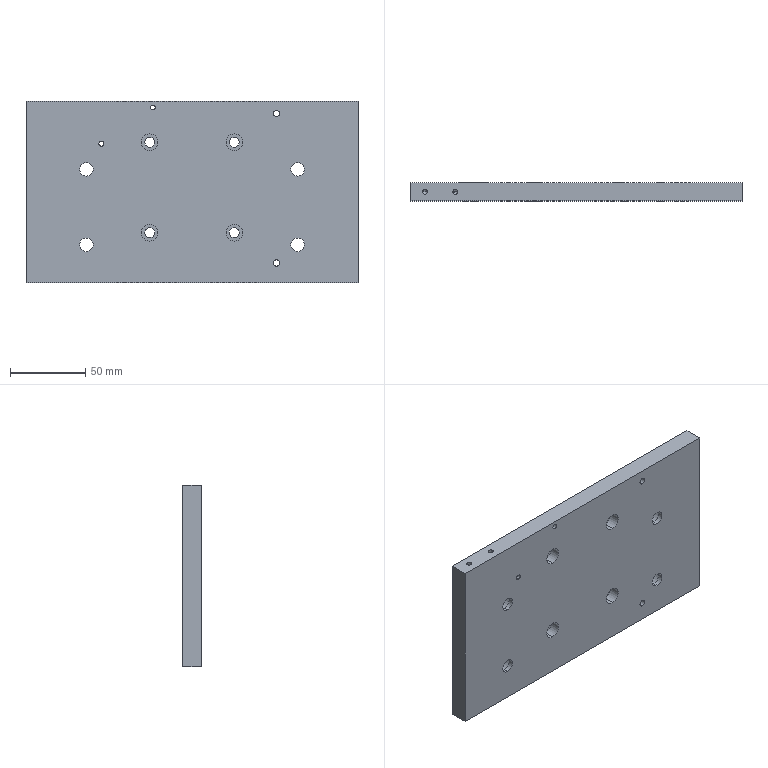Part | SolidWorks | features HoleWzd 6, 3DProfileFeature 3, Extrusion 1 | 1 solid | 74 faces | box 220 x 12 x 120 mm | volume 304867 mm3 | cylinder 50 | plane 14 | cone 10 | commonest cylinder face diameters 3.3 x8 6.6 x8 9 x8 11 x8 15 x8 5 x6